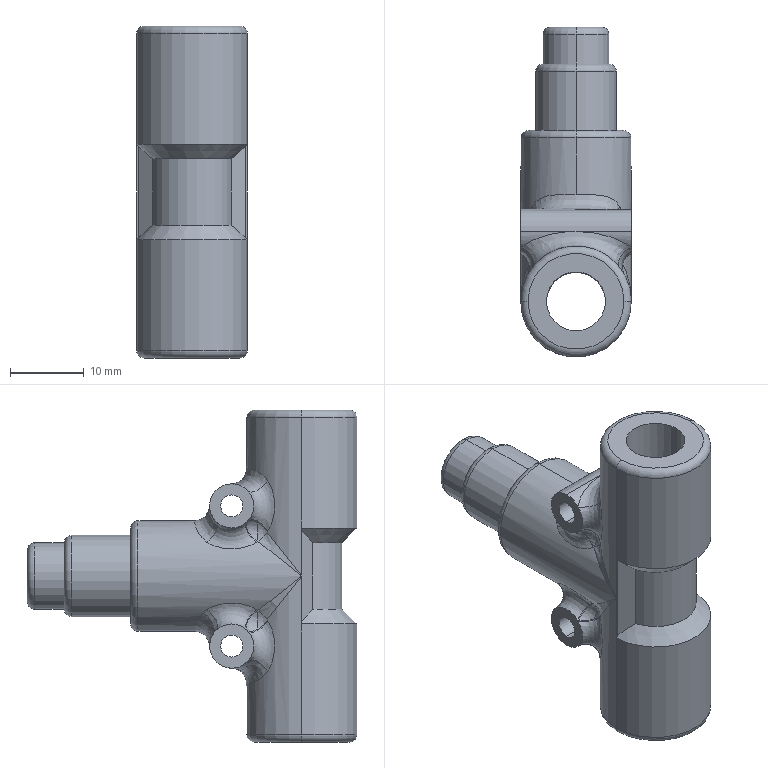Part | STEP file | Water-bath atomizer head | 1 solid | 87 faces | box 15 x 44.7 x 45 mm | volume 9906 mm3 | spline 28 | cylinder 27 | plane 12 | torus 10 | sphere 8 | cone 2 | commonest cylinder face diameters 6 x8 15 x6 3 x4 11 x3 2 x2 8 x2